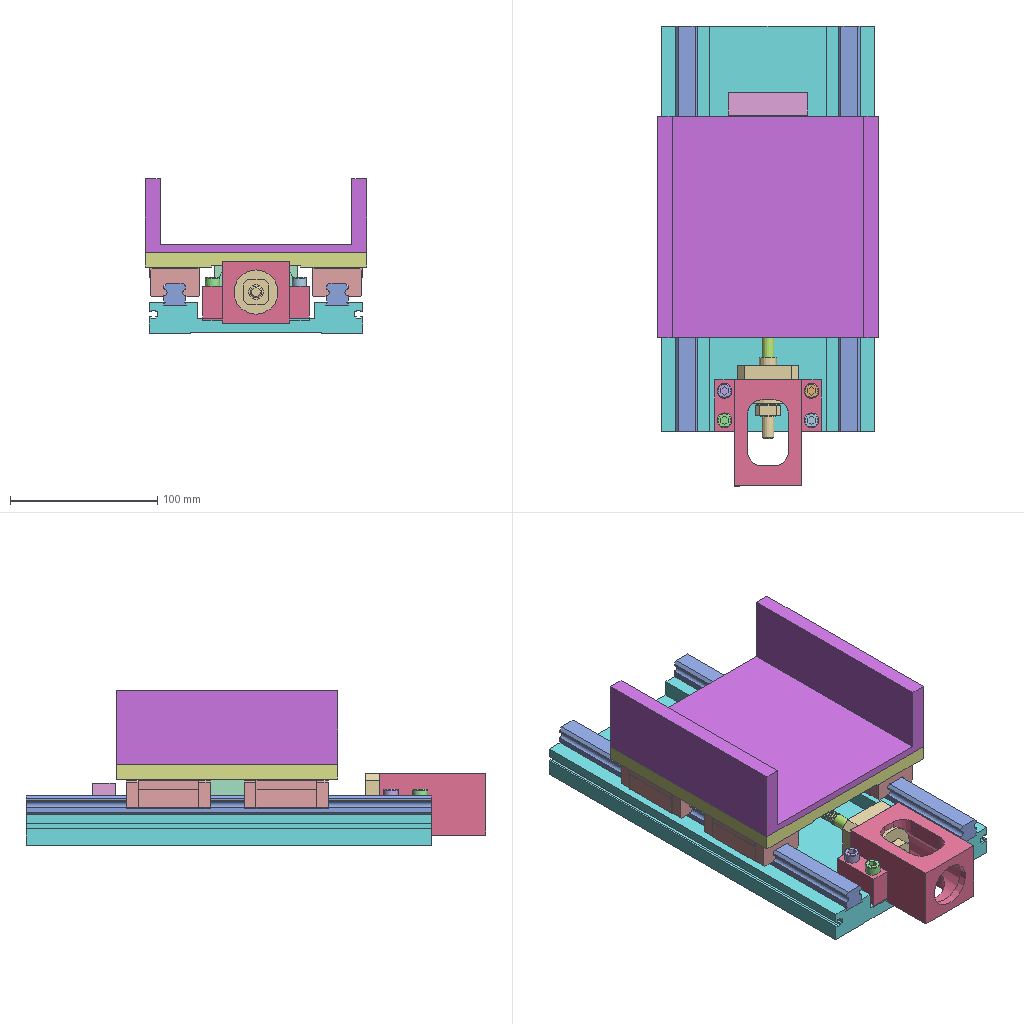Assembly | NX | 12 different items | 16 placed | box 150 x 312 x 105 mm
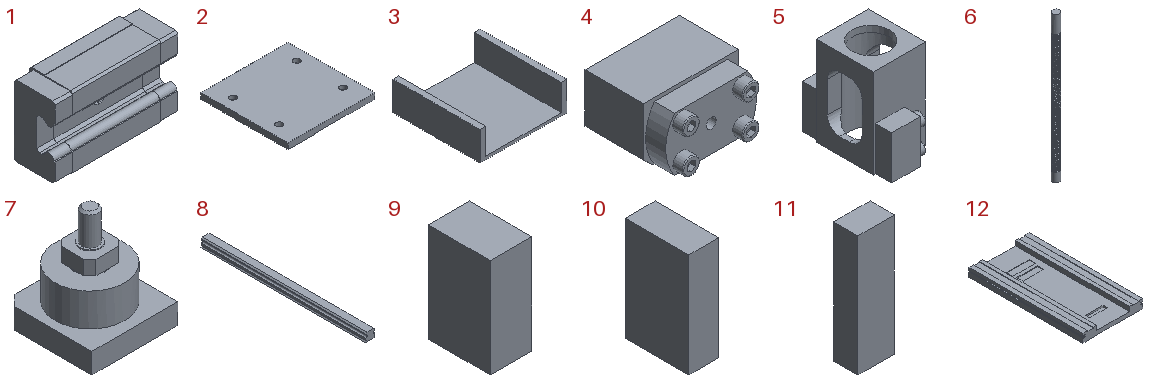Parts list (item | quantity | size | volume | features):
1 | x4 | 57 x 20 x 34 mm | 30744 mm3 | features BREP 1
2 | x1 | 150 x 150 x 10 mm | 212877 mm3 | features DATUM_CSYS 4, EXTRACT_BODY 3, EXTRUDE 3, SKETCH 3, Container 2, Geometry Instance 2, SUBTRACT 1
3 | x1 | 150 x 150 x 50 mm | 247500 mm3 | features DATUM_CSYS 2, EXTRUDE 1, SKETCH 1
4 | x1 | 56 x 53 x 34 mm | 80707 mm3 | features BREP 8, DATUM_CSYS 7, SKETCH 6, EXTRUDE 5, META 4, CHAMFER 1
5 | x1 | 42 x 72 x 72 mm | 82827 mm3 | features BREP 8, DATUM_CSYS 6, SKETCH 5, EXTRUDE 4, META 4, Container 1, EXTRACT_BODY 1, Geometry Instance 1, UNITE 1
6 | x1 | 8 x 8 x 170 mm | 7893 mm3 | features DATUM_CSYS 2, CYLINDER 1, HELIX 1, SKETCH 1, SKIN 1, SUBTRACT 1
7 | x1 | 42 x 43 x 55 mm | 35859 mm3 | features EXTRUDE 8, DATUM_CSYS 7, SKETCH 6, CHAMFER 3, OFFSET 1
8 | x2 | 16 x 275 x 14.5 mm | 53913 mm3 | features DATUM_CSYS 2, EXTRUDE 1, OFFSET 1, SKETCH 1
9 | x1 | 10 x 15 x 24 mm | 3600 mm3 | features BLOCK 1, DATUM_CSYS 1
10 | x1 | 15.5 x 33 x 54 mm | 25530 mm3 | features DATUM_CSYS 2, BLOCK 1, EXTRUDE 1, SKETCH 1
11 | x1 | 15 x 10 x 50 mm | 7500 mm3 | features BLOCK 1, DATUM_CSYS 1
12 | x1 | 145 x 275 x 21 mm | 550658 mm3 | features DATUM_CSYS 5, EXTRUDE 5, EXTRACT_BODY 4, SKETCH 4, Container 1, Geometry Instance 1, MOVE_FACE 1, SUBTRACT 1